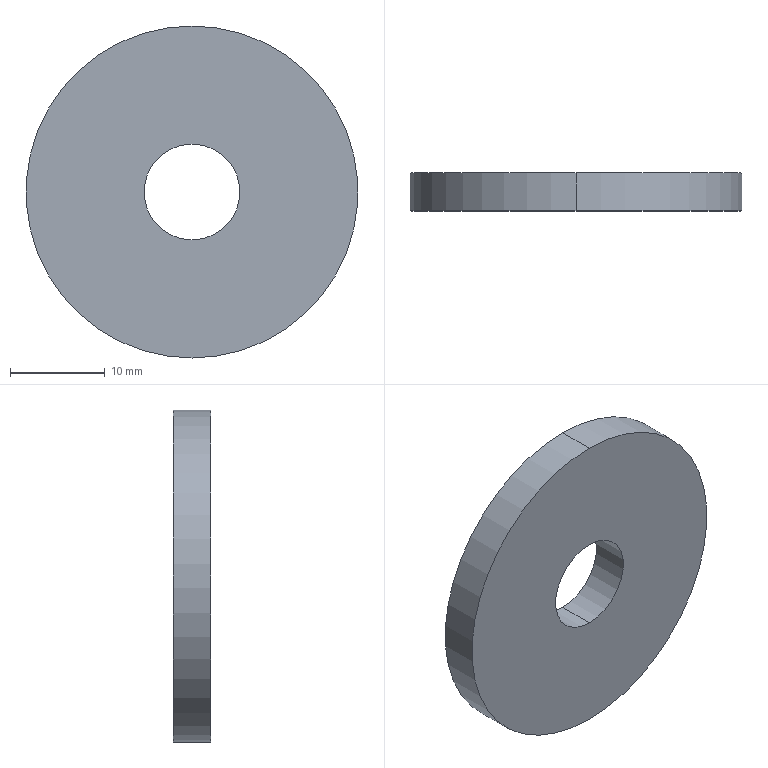Part | STEP file | 1 solid | 6 faces | box 35 x 4 x 35 mm | volume 3528 mm3 | cylinder 4 | plane 2 | commonest cylinder face diameters 10.1 x2 35 x2
STEP:
#1=CARTESIAN_POINT('',(0.,0.,0.));
#2=DIRECTION('',(0.,0.,1.));
#3=DIRECTION('',(1.,0.,0.));
#4=AXIS2_PLACEMENT_3D('',#1,#2,#3);
#5=CARTESIAN_POINT('',(0.,4.,-5.05));
#6=VERTEX_POINT('',#5);
#7=CARTESIAN_POINT('',(0.,0.,-5.05));
#8=VERTEX_POINT('',#7);
#9=CARTESIAN_POINT('',(0.,4.,-5.05));
#10=DIRECTION('',(0.,-1.,0.));
#11=VECTOR('',#10,1.);
#12=LINE('',#9,#11);
#13=CARTESIAN_POINT('',(0.,4.,0.));
#14=DIRECTION('',(0.,-1.,0.));
#15=DIRECTION('',(0.,0.,-1.));
#16=AXIS2_PLACEMENT_3D('',#13,#14,#15);
#17=CYLINDRICAL_SURFACE('',#16,5.05);
#18=CARTESIAN_POINT('',(6.283,0.));
#19=DIRECTION('',(0.,1.));
#20=VECTOR('',#19,1.);
#21=LINE('',#18,#20);
#22=(GEOMETRIC_REPRESENTATION_CONTEXT(2)PARAMETRIC_REPRESENTATION_CONTEXT()REPRESENTATION_CONTEXT('',''));
#23=DEFINITIONAL_REPRESENTATION('',(#21),#22);
#24=PCURVE('',#17,#23);
#25=CARTESIAN_POINT('',(0.,4.,0.));
#26=DIRECTION('',(0.,-1.,0.));
#27=DIRECTION('',(0.,0.,-1.));
#28=AXIS2_PLACEMENT_3D('',#25,#26,#27);
#29=CYLINDRICAL_SURFACE('',#28,5.05);
#30=CARTESIAN_POINT('',(0.,0.));
#31=DIRECTION('',(0.,1.));
#32=VECTOR('',#31,1.);
#33=LINE('',#30,#32);
#34=(GEOMETRIC_REPRESENTATION_CONTEXT(2)PARAMETRIC_REPRESENTATION_CONTEXT()REPRESENTATION_CONTEXT('',''));
#35=DEFINITIONAL_REPRESENTATION('',(#33),#34);
#36=PCURVE('',#29,#35);
#37=SURFACE_CURVE('',#12,(#24,#36),.PCURVE_S1.);
#38=EDGE_CURVE('',#6,#8,#37,.T.);
#39=ORIENTED_EDGE('',*,*,#38,.T.);
#40=CARTESIAN_POINT('',(0.,0.,5.05));
#41=VERTEX_POINT('',#40);
#42=CARTESIAN_POINT('',(0.,0.,0.));
#43=DIRECTION('',(0.,1.,0.));
#44=DIRECTION('',(0.,0.,1.));
#45=AXIS2_PLACEMENT_3D('',#42,#43,#44);
#46=CIRCLE('',#45,5.05);
#47=CARTESIAN_POINT('',(9.425,4.));
#48=DIRECTION('',(-1.,0.));
#49=VECTOR('',#48,1.);
#50=LINE('',#47,#49);
#51=(GEOMETRIC_REPRESENTATION_CONTEXT(2)PARAMETRIC_REPRESENTATION_CONTEXT()REPRESENTATION_CONTEXT('',''));
#52=DEFINITIONAL_REPRESENTATION('',(#50),#51);
#53=PCURVE('',#17,#52);
#54=CARTESIAN_POINT('',(0.,0.,0.));
#55=DIRECTION('',(0.,1.,0.));
#56=DIRECTION('',(0.,0.,1.));
#57=AXIS2_PLACEMENT_3D('',#54,#55,#56);
#58=PLANE('',#57);
#59=CARTESIAN_POINT('',(0.,0.));
#60=DIRECTION('',(1.,0.));
#61=AXIS2_PLACEMENT_2D('',#59,#60);
#62=CIRCLE('',#61,5.05);
#63=(GEOMETRIC_REPRESENTATION_CONTEXT(2)PARAMETRIC_REPRESENTATION_CONTEXT()REPRESENTATION_CONTEXT('',''));
#64=DEFINITIONAL_REPRESENTATION('',(#62),#63);
#65=PCURVE('',#58,#64);
#66=SURFACE_CURVE('',#46,(#53,#65),.PCURVE_S1.);
#67=EDGE_CURVE('',#8,#41,#66,.T.);
#68=ORIENTED_EDGE('',*,*,#67,.T.);
#69=CARTESIAN_POINT('',(0.,4.,5.05));
#70=VERTEX_POINT('',#69);
#71=CARTESIAN_POINT('',(0.,4.,5.05));
#72=DIRECTION('',(0.,-1.,0.));
#73=VECTOR('',#72,1.);
#74=LINE('',#71,#73);
#75=CARTESIAN_POINT('',(3.142,0.));
#76=DIRECTION('',(0.,1.));
#77=VECTOR('',#76,1.);
#78=LINE('',#75,#77);
#79=(GEOMETRIC_REPRESENTATION_CONTEXT(2)PARAMETRIC_REPRESENTATION_CONTEXT()REPRESENTATION_CONTEXT('',''));
#80=DEFINITIONAL_REPRESENTATION('',(#78),#79);
#81=PCURVE('',#17,#80);
#82=CARTESIAN_POINT('',(3.142,0.));
#83=DIRECTION('',(0.,1.));
#84=VECTOR('',#83,1.);
#85=LINE('',#82,#84);
#86=(GEOMETRIC_REPRESENTATION_CONTEXT(2)PARAMETRIC_REPRESENTATION_CONTEXT()REPRESENTATION_CONTEXT('',''));
#87=DEFINITIONAL_REPRESENTATION('',(#85),#86);
#88=PCURVE('',#29,#87);
#89=SURFACE_CURVE('',#74,(#81,#88),.PCURVE_S1.);
#90=EDGE_CURVE('',#70,#41,#89,.T.);
#91=ORIENTED_EDGE('',*,*,#90,.F.);
#92=CARTESIAN_POINT('',(0.,4.,0.));
#93=DIRECTION('',(0.,1.,0.));
#94=DIRECTION('',(0.,0.,1.));
#95=AXIS2_PLACEMENT_3D('',#92,#93,#94);
#96=CIRCLE('',#95,5.05);
#97=CARTESIAN_POINT('',(9.425,0.));
#98=DIRECTION('',(-1.,0.));
#99=VECTOR('',#98,1.);
#100=LINE('',#97,#99);
#101=(GEOMETRIC_REPRESENTATION_CONTEXT(2)PARAMETRIC_REPRESENTATION_CONTEXT()REPRESENTATION_CONTEXT('',''));
#102=DEFINITIONAL_REPRESENTATION('',(#100),#101);
#103=PCURVE('',#17,#102);
#104=CARTESIAN_POINT('',(0.,4.,0.));
#105=DIRECTION('',(0.,1.,0.));
#106=DIRECTION('',(0.,0.,1.));
#107=AXIS2_PLACEMENT_3D('',#104,#105,#106);
#108=PLANE('',#107);
#109=CARTESIAN_POINT('',(0.,0.));
#110=DIRECTION('',(1.,0.));
#111=AXIS2_PLACEMENT_2D('',#109,#110);
#112=CIRCLE('',#111,5.05);
#113=(GEOMETRIC_REPRESENTATION_CONTEXT(2)PARAMETRIC_REPRESENTATION_CONTEXT()REPRESENTATION_CONTEXT('',''));
#114=DEFINITIONAL_REPRESENTATION('',(#112),#113);
#115=PCURVE('',#108,#114);
#116=SURFACE_CURVE('',#96,(#103,#115),.PCURVE_S1.);
#117=EDGE_CURVE('',#6,#70,#116,.T.);
#118=ORIENTED_EDGE('',*,*,#117,.F.);
#119=EDGE_LOOP('',(#39,#68,#91,#118));
#120=FACE_BOUND('',#119,.F.);
#121=ADVANCED_FACE('',(#120),#17,.F.);
#122=CARTESIAN_POINT('',(0.,4.,17.5));
#123=VERTEX_POINT('',#122);
#124=CARTESIAN_POINT('',(0.,4.,-17.5));
#125=VERTEX_POINT('',#124);
#126=CARTESIAN_POINT('',(0.,4.,0.));
#127=DIRECTION('',(0.,1.,0.));
#128=DIRECTION('',(0.,0.,1.));
#129=AXIS2_PLACEMENT_3D('',#126,#127,#128);
#130=CIRCLE('',#129,17.5);
#131=CARTESIAN_POINT('',(0.,4.,0.));
#132=DIRECTION('',(0.,-1.,0.));
#133=DIRECTION('',(0.,0.,-1.));
#134=AXIS2_PLACEMENT_3D('',#131,#132,#133);
#135=CYLINDRICAL_SURFACE('',#134,17.5);
#136=CARTESIAN_POINT('',(3.142,0.));
#137=DIRECTION('',(-1.,0.));
#138=VECTOR('',#137,1.);
#139=LINE('',#136,#138);
#140=(GEOMETRIC_REPRESENTATION_CONTEXT(2)PARAMETRIC_REPRESENTATION_CONTEXT()REPRESENTATION_CONTEXT('',''));
#141=DEFINITIONAL_REPRESENTATION('',(#139),#140);
#142=PCURVE('',#135,#141);
#143=CARTESIAN_POINT('',(0.,0.));
#144=DIRECTION('',(1.,0.));
#145=AXIS2_PLACEMENT_2D('',#143,#144);
#146=CIRCLE('',#145,17.5);
#147=(GEOMETRIC_REPRESENTATION_CONTEXT(2)PARAMETRIC_REPRESENTATION_CONTEXT()REPRESENTATION_CONTEXT('',''));
#148=DEFINITIONAL_REPRESENTATION('',(#146),#147);
#149=PCURVE('',#108,#148);
#150=SURFACE_CURVE('',#130,(#142,#149),.PCURVE_S1.);
#151=EDGE_CURVE('',#123,#125,#150,.T.);
#152=ORIENTED_EDGE('',*,*,#151,.F.);
#153=CARTESIAN_POINT('',(0.,0.,17.5));
#154=VERTEX_POINT('',#153);
#155=CARTESIAN_POINT('',(0.,4.,17.5));
#156=DIRECTION('',(0.,-1.,0.));
#157=VECTOR('',#156,1.);
#158=LINE('',#155,#157);
#159=CARTESIAN_POINT('',(3.142,0.));
#160=DIRECTION('',(0.,1.));
#161=VECTOR('',#160,1.);
#162=LINE('',#159,#161);
#163=(GEOMETRIC_REPRESENTATION_CONTEXT(2)PARAMETRIC_REPRESENTATION_CONTEXT()REPRESENTATION_CONTEXT('',''));
#164=DEFINITIONAL_REPRESENTATION('',(#162),#163);
#165=PCURVE('',#135,#164);
#166=CARTESIAN_POINT('',(0.,4.,0.));
#167=DIRECTION('',(0.,-1.,0.));
#168=DIRECTION('',(0.,0.,-1.));
#169=AXIS2_PLACEMENT_3D('',#166,#167,#168);
#170=CYLINDRICAL_SURFACE('',#169,17.5);
#171=CARTESIAN_POINT('',(3.142,0.));
#172=DIRECTION('',(0.,1.));
#173=VECTOR('',#172,1.);
#174=LINE('',#171,#173);
#175=(GEOMETRIC_REPRESENTATION_CONTEXT(2)PARAMETRIC_REPRESENTATION_CONTEXT()REPRESENTATION_CONTEXT('',''));
#176=DEFINITIONAL_REPRESENTATION('',(#174),#175);
#177=PCURVE('',#170,#176);
#178=SURFACE_CURVE('',#158,(#165,#177),.PCURVE_S1.);
#179=EDGE_CURVE('',#123,#154,#178,.T.);
#180=ORIENTED_EDGE('',*,*,#179,.T.);
#181=CARTESIAN_POINT('',(0.,0.,-17.5));
#182=VERTEX_POINT('',#181);
#183=CARTESIAN_POINT('',(0.,0.,0.));
#184=DIRECTION('',(0.,1.,0.));
#185=DIRECTION('',(0.,0.,1.));
#186=AXIS2_PLACEMENT_3D('',#183,#184,#185);
#187=CIRCLE('',#186,17.5);
#188=CARTESIAN_POINT('',(3.142,4.));
#189=DIRECTION('',(-1.,0.));
#190=VECTOR('',#189,1.);
#191=LINE('',#188,#190);
#192=(GEOMETRIC_REPRESENTATION_CONTEXT(2)PARAMETRIC_REPRESENTATION_CONTEXT()REPRESENTATION_CONTEXT('',''));
#193=DEFINITIONAL_REPRESENTATION('',(#191),#192);
#194=PCURVE('',#135,#193);
#195=CARTESIAN_POINT('',(0.,0.));
#196=DIRECTION('',(1.,0.));
#197=AXIS2_PLACEMENT_2D('',#195,#196);
#198=CIRCLE('',#197,17.5);
#199=(GEOMETRIC_REPRESENTATION_CONTEXT(2)PARAMETRIC_REPRESENTATION_CONTEXT()REPRESENTATION_CONTEXT('',''));
#200=DEFINITIONAL_REPRESENTATION('',(#198),#199);
#201=PCURVE('',#58,#200);
#202=SURFACE_CURVE('',#187,(#194,#201),.PCURVE_S1.);
#203=EDGE_CURVE('',#154,#182,#202,.T.);
#204=ORIENTED_EDGE('',*,*,#203,.T.);
#205=CARTESIAN_POINT('',(0.,4.,-17.5));
#206=DIRECTION('',(0.,-1.,0.));
#207=VECTOR('',#206,1.);
#208=LINE('',#205,#207);
#209=CARTESIAN_POINT('',(0.,0.));
#210=DIRECTION('',(0.,1.));
#211=VECTOR('',#210,1.);
#212=LINE('',#209,#211);
#213=(GEOMETRIC_REPRESENTATION_CONTEXT(2)PARAMETRIC_REPRESENTATION_CONTEXT()REPRESENTATION_CONTEXT('',''));
#214=DEFINITIONAL_REPRESENTATION('',(#212),#213);
#215=PCURVE('',#135,#214);
#216=CARTESIAN_POINT('',(6.283,0.));
#217=DIRECTION('',(0.,1.));
#218=VECTOR('',#217,1.);
#219=LINE('',#216,#218);
#220=(GEOMETRIC_REPRESENTATION_CONTEXT(2)PARAMETRIC_REPRESENTATION_CONTEXT()REPRESENTATION_CONTEXT('',''));
#221=DEFINITIONAL_REPRESENTATION('',(#219),#220);
#222=PCURVE('',#170,#221);
#223=SURFACE_CURVE('',#208,(#215,#222),.PCURVE_S1.);
#224=EDGE_CURVE('',#125,#182,#223,.T.);
#225=ORIENTED_EDGE('',*,*,#224,.F.);
#226=EDGE_LOOP('',(#152,#180,#204,#225));
#227=FACE_BOUND('',#226,.T.);
#228=ADVANCED_FACE('',(#227),#135,.T.);
#229=CARTESIAN_POINT('',(0.,4.,0.));
#230=DIRECTION('',(0.,1.,0.));
#231=DIRECTION('',(0.,0.,1.));
#232=AXIS2_PLACEMENT_3D('',#229,#230,#231);
#233=CIRCLE('',#232,17.5);
#234=CARTESIAN_POINT('',(0.,0.));
#235=DIRECTION('',(1.,0.));
#236=AXIS2_PLACEMENT_2D('',#234,#235);
#237=CIRCLE('',#236,17.5);
#238=(GEOMETRIC_REPRESENTATION_CONTEXT(2)PARAMETRIC_REPRESENTATION_CONTEXT()REPRESENTATION_CONTEXT('',''));
#239=DEFINITIONAL_REPRESENTATION('',(#237),#238);
#240=PCURVE('',#108,#239);
#241=CARTESIAN_POINT('',(9.425,0.));
#242=DIRECTION('',(-1.,0.));
#243=VECTOR('',#242,1.);
#244=LINE('',#241,#243);
#245=(GEOMETRIC_REPRESENTATION_CONTEXT(2)PARAMETRIC_REPRESENTATION_CONTEXT()REPRESENTATION_CONTEXT('',''));
#246=DEFINITIONAL_REPRESENTATION('',(#244),#245);
#247=PCURVE('',#170,#246);
#248=SURFACE_CURVE('',#233,(#240,#247),.PCURVE_S1.);
#249=EDGE_CURVE('',#125,#123,#248,.T.);
#250=ORIENTED_EDGE('',*,*,#249,.T.);
#251=ORIENTED_EDGE('',*,*,#151,.T.);
#252=EDGE_LOOP('',(#250,#251));
#253=FACE_BOUND('',#252,.T.);
#254=ORIENTED_EDGE('',*,*,#117,.F.);
#255=CARTESIAN_POINT('',(0.,4.,0.));
#256=DIRECTION('',(0.,1.,0.));
#257=DIRECTION('',(0.,0.,1.));
#258=AXIS2_PLACEMENT_3D('',#255,#256,#257);
#259=CIRCLE('',#258,5.05);
#260=CARTESIAN_POINT('',(0.,0.));
#261=DIRECTION('',(1.,0.));
#262=AXIS2_PLACEMENT_2D('',#260,#261);
#263=CIRCLE('',#262,5.05);
#264=(GEOMETRIC_REPRESENTATION_CONTEXT(2)PARAMETRIC_REPRESENTATION_CONTEXT()REPRESENTATION_CONTEXT('',''));
#265=DEFINITIONAL_REPRESENTATION('',(#263),#264);
#266=PCURVE('',#108,#265);
#267=CARTESIAN_POINT('',(3.142,0.));
#268=DIRECTION('',(-1.,0.));
#269=VECTOR('',#268,1.);
#270=LINE('',#267,#269);
#271=(GEOMETRIC_REPRESENTATION_CONTEXT(2)PARAMETRIC_REPRESENTATION_CONTEXT()REPRESENTATION_CONTEXT('',''));
#272=DEFINITIONAL_REPRESENTATION('',(#270),#271);
#273=PCURVE('',#29,#272);
#274=SURFACE_CURVE('',#259,(#266,#273),.PCURVE_S1.);
#275=EDGE_CURVE('',#70,#6,#274,.T.);
#276=ORIENTED_EDGE('',*,*,#275,.F.);
#277=EDGE_LOOP('',(#254,#276));
#278=FACE_BOUND('',#277,.T.);
#279=ADVANCED_FACE('',(#253,#278),#108,.T.);
#280=CARTESIAN_POINT('',(0.,0.,0.));
#281=DIRECTION('',(0.,1.,0.));
#282=DIRECTION('',(0.,0.,1.));
#283=AXIS2_PLACEMENT_3D('',#280,#281,#282);
#284=CIRCLE('',#283,17.5);
#285=CARTESIAN_POINT('',(0.,0.));
#286=DIRECTION('',(1.,0.));
#287=AXIS2_PLACEMENT_2D('',#285,#286);
#288=CIRCLE('',#287,17.5);
#289=(GEOMETRIC_REPRESENTATION_CONTEXT(2)PARAMETRIC_REPRESENTATION_CONTEXT()REPRESENTATION_CONTEXT('',''));
#290=DEFINITIONAL_REPRESENTATION('',(#288),#289);
#291=PCURVE('',#58,#290);
#292=CARTESIAN_POINT('',(9.425,4.));
#293=DIRECTION('',(-1.,0.));
#294=VECTOR('',#293,1.);
#295=LINE('',#292,#294);
#296=(GEOMETRIC_REPRESENTATION_CONTEXT(2)PARAMETRIC_REPRESENTATION_CONTEXT()REPRESENTATION_CONTEXT('',''));
#297=DEFINITIONAL_REPRESENTATION('',(#295),#296);
#298=PCURVE('',#170,#297);
#299=SURFACE_CURVE('',#284,(#291,#298),.PCURVE_S1.);
#300=EDGE_CURVE('',#182,#154,#299,.T.);
#301=ORIENTED_EDGE('',*,*,#300,.F.);
#302=ORIENTED_EDGE('',*,*,#203,.F.);
#303=EDGE_LOOP('',(#301,#302));
#304=FACE_BOUND('',#303,.T.);
#305=ORIENTED_EDGE('',*,*,#67,.T.);
#306=CARTESIAN_POINT('',(0.,0.,0.));
#307=DIRECTION('',(0.,1.,0.));
#308=DIRECTION('',(0.,0.,1.));
#309=AXIS2_PLACEMENT_3D('',#306,#307,#308);
#310=CIRCLE('',#309,5.05);
#311=CARTESIAN_POINT('',(0.,0.));
#312=DIRECTION('',(1.,0.));
#313=AXIS2_PLACEMENT_2D('',#311,#312);
#314=CIRCLE('',#313,5.05);
#315=(GEOMETRIC_REPRESENTATION_CONTEXT(2)PARAMETRIC_REPRESENTATION_CONTEXT()REPRESENTATION_CONTEXT('',''));
#316=DEFINITIONAL_REPRESENTATION('',(#314),#315);
#317=PCURVE('',#58,#316);
#318=CARTESIAN_POINT('',(3.142,4.));
#319=DIRECTION('',(-1.,0.));
#320=VECTOR('',#319,1.);
#321=LINE('',#318,#320);
#322=(GEOMETRIC_REPRESENTATION_CONTEXT(2)PARAMETRIC_REPRESENTATION_CONTEXT()REPRESENTATION_CONTEXT('',''));
#323=DEFINITIONAL_REPRESENTATION('',(#321),#322);
#324=PCURVE('',#29,#323);
#325=SURFACE_CURVE('',#310,(#317,#324),.PCURVE_S1.);
#326=EDGE_CURVE('',#41,#8,#325,.T.);
#327=ORIENTED_EDGE('',*,*,#326,.T.);
#328=EDGE_LOOP('',(#305,#327));
#329=FACE_BOUND('',#328,.T.);
#330=ADVANCED_FACE('',(#304,#329),#58,.F.);
#331=ORIENTED_EDGE('',*,*,#179,.F.);
#332=ORIENTED_EDGE('',*,*,#249,.F.);
#333=ORIENTED_EDGE('',*,*,#224,.T.);
#334=ORIENTED_EDGE('',*,*,#300,.T.);
#335=EDGE_LOOP('',(#331,#332,#333,#334));
#336=FACE_BOUND('',#335,.T.);
#337=ADVANCED_FACE('',(#336),#170,.T.);
#338=ORIENTED_EDGE('',*,*,#326,.T.);
#339=ORIENTED_EDGE('',*,*,#38,.F.);
#340=ORIENTED_EDGE('',*,*,#275,.F.);
#341=ORIENTED_EDGE('',*,*,#90,.T.);
#342=EDGE_LOOP('',(#338,#339,#340,#341));
#343=FACE_BOUND('',#342,.F.);
#344=ADVANCED_FACE('',(#343),#29,.F.);
#345=CLOSED_SHELL('',(#121,#228,#279,#330,#337,#344));
#346=MANIFOLD_SOLID_BREP('',#345);
#347=(LENGTH_UNIT()NAMED_UNIT(*)SI_UNIT(.MILLI.,.METRE.));
#348=UNCERTAINTY_MEASURE_WITH_UNIT(LENGTH_MEASURE(0.0000001),#347,'','');
#349=(NAMED_UNIT(*)PLANE_ANGLE_UNIT()SI_UNIT($,.RADIAN.));
#350=(NAMED_UNIT(*)SI_UNIT($,.STERADIAN.)SOLID_ANGLE_UNIT());
#351=(GEOMETRIC_REPRESENTATION_CONTEXT(3)GLOBAL_UNCERTAINTY_ASSIGNED_CONTEXT((#348))GLOBAL_UNIT_ASSIGNED_CONTEXT((#347,#349,#350))REPRESENTATION_CONTEXT('',''));
#352=ADVANCED_BREP_SHAPE_REPRESENTATION('',(#4,#346),#351);